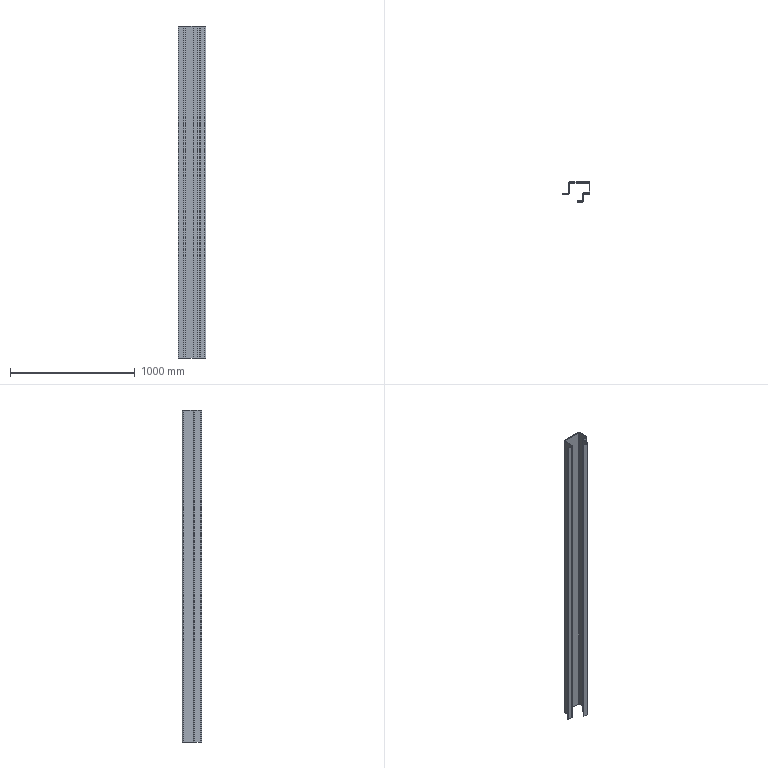Part | SolidWorks | features Extrusion 1 | 1 solid | 30 faces | box 224 x 158 x 2660 mm | volume 8679415 mm3 | plane 18 | cylinder 12 | commonest cylinder face diameters 12 x6 24 x6
STEP:
#1=CARTESIAN_POINT('',(-59.,158.,0.));
#2=VERTEX_POINT('',#1);
#3=CARTESIAN_POINT('',(-71.,146.,0.));
#4=VERTEX_POINT('',#3);
#5=CARTESIAN_POINT('',(-59.,146.,0.));
#6=DIRECTION('',(0.,0.,1.));
#7=DIRECTION('',(1.,0.,0.));
#8=AXIS2_PLACEMENT_3D('',#5,#6,#7);
#9=CIRCLE('',#8,12.);
#10=EDGE_CURVE('',#2,#4,#9,.T.);
#11=ORIENTED_EDGE('',*,*,#10,.T.);
#12=CARTESIAN_POINT('',(-71.,146.,2660.));
#13=VERTEX_POINT('',#12);
#14=CARTESIAN_POINT('',(-71.,146.,2660.));
#15=DIRECTION('',(0.,0.,-1.));
#16=VECTOR('',#15,1000.);
#17=LINE('',#14,#16);
#18=EDGE_CURVE('',#13,#4,#17,.T.);
#19=ORIENTED_EDGE('',*,*,#18,.F.);
#20=CARTESIAN_POINT('',(-59.,158.,2660.));
#21=VERTEX_POINT('',#20);
#22=CARTESIAN_POINT('',(-59.,146.,2660.));
#23=DIRECTION('',(0.,0.,1.));
#24=DIRECTION('',(1.,0.,0.));
#25=AXIS2_PLACEMENT_3D('',#22,#23,#24);
#26=CIRCLE('',#25,12.);
#27=EDGE_CURVE('',#21,#13,#26,.T.);
#28=ORIENTED_EDGE('',*,*,#27,.F.);
#29=CARTESIAN_POINT('',(-59.,158.,2660.));
#30=DIRECTION('',(0.,0.,-1.));
#31=VECTOR('',#30,1000.);
#32=LINE('',#29,#31);
#33=EDGE_CURVE('',#21,#2,#32,.T.);
#34=ORIENTED_EDGE('',*,*,#33,.T.);
#35=EDGE_LOOP('',(#11,#19,#28,#34));
#36=FACE_OUTER_BOUND('',#35,.T.);
#37=CARTESIAN_POINT('',(-59.,146.,2660.));
#38=DIRECTION('',(0.,0.,-1.));
#39=DIRECTION('',(-1.,0.,0.));
#40=AXIS2_PLACEMENT_3D('',#37,#38,#39);
#41=CYLINDRICAL_SURFACE('',#40,12.);
#42=ADVANCED_FACE('',(#36),#41,.T.);
#43=CARTESIAN_POINT('',(-71.,70.,0.));
#44=VERTEX_POINT('',#43);
#45=CARTESIAN_POINT('',(-71.,146.,0.));
#46=DIRECTION('',(0.,-1.,0.));
#47=VECTOR('',#46,1000.);
#48=LINE('',#45,#47);
#49=EDGE_CURVE('',#4,#44,#48,.T.);
#50=ORIENTED_EDGE('',*,*,#49,.T.);
#51=CARTESIAN_POINT('',(-71.,70.,2660.));
#52=VERTEX_POINT('',#51);
#53=CARTESIAN_POINT('',(-71.,70.,2660.));
#54=DIRECTION('',(0.,0.,-1.));
#55=VECTOR('',#54,1000.);
#56=LINE('',#53,#55);
#57=EDGE_CURVE('',#52,#44,#56,.T.);
#58=ORIENTED_EDGE('',*,*,#57,.F.);
#59=CARTESIAN_POINT('',(-71.,146.,2660.));
#60=DIRECTION('',(0.,-1.,0.));
#61=VECTOR('',#60,1000.);
#62=LINE('',#59,#61);
#63=EDGE_CURVE('',#13,#52,#62,.T.);
#64=ORIENTED_EDGE('',*,*,#63,.F.);
#65=ORIENTED_EDGE('',*,*,#18,.T.);
#66=EDGE_LOOP('',(#50,#58,#64,#65));
#67=FACE_OUTER_BOUND('',#66,.T.);
#68=CARTESIAN_POINT('',(-71.,146.,2660.));
#69=DIRECTION('',(1.,0.,0.));
#70=DIRECTION('',(0.,1.,0.));
#71=AXIS2_PLACEMENT_3D('',#68,#69,#70);
#72=PLANE('',#71);
#73=ADVANCED_FACE('',(#67),#72,.F.);
#74=CARTESIAN_POINT('',(-77.,64.,0.));
#75=VERTEX_POINT('',#74);
#76=CARTESIAN_POINT('',(-77.,70.,0.));
#77=DIRECTION('',(0.,0.,-1.));
#78=DIRECTION('',(1.,0.,0.));
#79=AXIS2_PLACEMENT_3D('',#76,#77,#78);
#80=CIRCLE('',#79,6.);
#81=EDGE_CURVE('',#44,#75,#80,.T.);
#82=ORIENTED_EDGE('',*,*,#81,.T.);
#83=CARTESIAN_POINT('',(-77.,64.,2660.));
#84=VERTEX_POINT('',#83);
#85=CARTESIAN_POINT('',(-77.,64.,2660.));
#86=DIRECTION('',(0.,0.,-1.));
#87=VECTOR('',#86,1000.);
#88=LINE('',#85,#87);
#89=EDGE_CURVE('',#84,#75,#88,.T.);
#90=ORIENTED_EDGE('',*,*,#89,.F.);
#91=CARTESIAN_POINT('',(-77.,70.,2660.));
#92=DIRECTION('',(0.,0.,-1.));
#93=DIRECTION('',(1.,0.,0.));
#94=AXIS2_PLACEMENT_3D('',#91,#92,#93);
#95=CIRCLE('',#94,6.);
#96=EDGE_CURVE('',#52,#84,#95,.T.);
#97=ORIENTED_EDGE('',*,*,#96,.F.);
#98=ORIENTED_EDGE('',*,*,#57,.T.);
#99=EDGE_LOOP('',(#82,#90,#97,#98));
#100=FACE_OUTER_BOUND('',#99,.T.);
#101=CARTESIAN_POINT('',(-77.,70.,2660.));
#102=DIRECTION('',(0.,0.,-1.));
#103=DIRECTION('',(-1.,0.,0.));
#104=AXIS2_PLACEMENT_3D('',#101,#102,#103);
#105=CYLINDRICAL_SURFACE('',#104,6.);
#106=ADVANCED_FACE('',(#100),#105,.F.);
#107=CARTESIAN_POINT('',(-121.,64.,0.));
#108=VERTEX_POINT('',#107);
#109=CARTESIAN_POINT('',(-77.,64.,0.));
#110=DIRECTION('',(-1.,0.,0.));
#111=VECTOR('',#110,1000.);
#112=LINE('',#109,#111);
#113=EDGE_CURVE('',#75,#108,#112,.T.);
#114=ORIENTED_EDGE('',*,*,#113,.T.);
#115=CARTESIAN_POINT('',(-121.,64.,2660.));
#116=VERTEX_POINT('',#115);
#117=CARTESIAN_POINT('',(-121.,64.,2660.));
#118=DIRECTION('',(0.,0.,-1.));
#119=VECTOR('',#118,1000.);
#120=LINE('',#117,#119);
#121=EDGE_CURVE('',#116,#108,#120,.T.);
#122=ORIENTED_EDGE('',*,*,#121,.F.);
#123=CARTESIAN_POINT('',(-77.,64.,2660.));
#124=DIRECTION('',(-1.,0.,0.));
#125=VECTOR('',#124,1000.);
#126=LINE('',#123,#125);
#127=EDGE_CURVE('',#84,#116,#126,.T.);
#128=ORIENTED_EDGE('',*,*,#127,.F.);
#129=ORIENTED_EDGE('',*,*,#89,.T.);
#130=EDGE_LOOP('',(#114,#122,#128,#129));
#131=FACE_OUTER_BOUND('',#130,.T.);
#132=CARTESIAN_POINT('',(-77.,64.,2660.));
#133=DIRECTION('',(0.,-1.,0.));
#134=DIRECTION('',(1.,0.,0.));
#135=AXIS2_PLACEMENT_3D('',#132,#133,#134);
#136=PLANE('',#135);
#137=ADVANCED_FACE('',(#131),#136,.F.);
#138=CARTESIAN_POINT('',(-121.,58.,0.));
#139=VERTEX_POINT('',#138);
#140=CARTESIAN_POINT('',(-121.,64.,0.));
#141=DIRECTION('',(0.,-1.,0.));
#142=VECTOR('',#141,1000.);
#143=LINE('',#140,#142);
#144=EDGE_CURVE('',#108,#139,#143,.T.);
#145=ORIENTED_EDGE('',*,*,#144,.T.);
#146=CARTESIAN_POINT('',(-121.,58.,2660.));
#147=VERTEX_POINT('',#146);
#148=CARTESIAN_POINT('',(-121.,58.,2660.));
#149=DIRECTION('',(0.,0.,-1.));
#150=VECTOR('',#149,1000.);
#151=LINE('',#148,#150);
#152=EDGE_CURVE('',#147,#139,#151,.T.);
#153=ORIENTED_EDGE('',*,*,#152,.F.);
#154=CARTESIAN_POINT('',(-121.,64.,2660.));
#155=DIRECTION('',(0.,-1.,0.));
#156=VECTOR('',#155,1000.);
#157=LINE('',#154,#156);
#158=EDGE_CURVE('',#116,#147,#157,.T.);
#159=ORIENTED_EDGE('',*,*,#158,.F.);
#160=ORIENTED_EDGE('',*,*,#121,.T.);
#161=EDGE_LOOP('',(#145,#153,#159,#160));
#162=FACE_OUTER_BOUND('',#161,.T.);
#163=CARTESIAN_POINT('',(-121.,64.,2660.));
#164=DIRECTION('',(1.,0.,0.));
#165=DIRECTION('',(0.,0.,-1.));
#166=AXIS2_PLACEMENT_3D('',#163,#164,#165);
#167=PLANE('',#166);
#168=ADVANCED_FACE('',(#162),#167,.F.);
#169=CARTESIAN_POINT('',(-77.,58.,0.));
#170=VERTEX_POINT('',#169);
#171=CARTESIAN_POINT('',(-121.,58.,0.));
#172=DIRECTION('',(1.,0.,0.));
#173=VECTOR('',#172,1000.);
#174=LINE('',#171,#173);
#175=EDGE_CURVE('',#139,#170,#174,.T.);
#176=ORIENTED_EDGE('',*,*,#175,.T.);
#177=CARTESIAN_POINT('',(-77.,58.,2660.));
#178=VERTEX_POINT('',#177);
#179=CARTESIAN_POINT('',(-77.,58.,2660.));
#180=DIRECTION('',(0.,0.,-1.));
#181=VECTOR('',#180,1000.);
#182=LINE('',#179,#181);
#183=EDGE_CURVE('',#178,#170,#182,.T.);
#184=ORIENTED_EDGE('',*,*,#183,.F.);
#185=CARTESIAN_POINT('',(-121.,58.,2660.));
#186=DIRECTION('',(1.,0.,0.));
#187=VECTOR('',#186,1000.);
#188=LINE('',#185,#187);
#189=EDGE_CURVE('',#147,#178,#188,.T.);
#190=ORIENTED_EDGE('',*,*,#189,.F.);
#191=ORIENTED_EDGE('',*,*,#152,.T.);
#192=EDGE_LOOP('',(#176,#184,#190,#191));
#193=FACE_OUTER_BOUND('',#192,.T.);
#194=CARTESIAN_POINT('',(-121.,58.,2660.));
#195=DIRECTION('',(0.,1.,0.));
#196=DIRECTION('',(0.,0.,1.));
#197=AXIS2_PLACEMENT_3D('',#194,#195,#196);
#198=PLANE('',#197);
#199=ADVANCED_FACE('',(#193),#198,.F.);
#200=CARTESIAN_POINT('',(-65.,70.,0.));
#201=VERTEX_POINT('',#200);
#202=CARTESIAN_POINT('',(-77.,70.,0.));
#203=DIRECTION('',(0.,0.,1.));
#204=DIRECTION('',(1.,0.,0.));
#205=AXIS2_PLACEMENT_3D('',#202,#203,#204);
#206=CIRCLE('',#205,12.);
#207=EDGE_CURVE('',#170,#201,#206,.T.);
#208=ORIENTED_EDGE('',*,*,#207,.T.);
#209=CARTESIAN_POINT('',(-65.,70.,2660.));
#210=VERTEX_POINT('',#209);
#211=CARTESIAN_POINT('',(-65.,70.,2660.));
#212=DIRECTION('',(0.,0.,-1.));
#213=VECTOR('',#212,1000.);
#214=LINE('',#211,#213);
#215=EDGE_CURVE('',#210,#201,#214,.T.);
#216=ORIENTED_EDGE('',*,*,#215,.F.);
#217=CARTESIAN_POINT('',(-77.,70.,2660.));
#218=DIRECTION('',(0.,0.,1.));
#219=DIRECTION('',(1.,0.,0.));
#220=AXIS2_PLACEMENT_3D('',#217,#218,#219);
#221=CIRCLE('',#220,12.);
#222=EDGE_CURVE('',#178,#210,#221,.T.);
#223=ORIENTED_EDGE('',*,*,#222,.F.);
#224=ORIENTED_EDGE('',*,*,#183,.T.);
#225=EDGE_LOOP('',(#208,#216,#223,#224));
#226=FACE_OUTER_BOUND('',#225,.T.);
#227=CARTESIAN_POINT('',(-77.,70.,2660.));
#228=DIRECTION('',(0.,0.,-1.));
#229=DIRECTION('',(-1.,0.,0.));
#230=AXIS2_PLACEMENT_3D('',#227,#228,#229);
#231=CYLINDRICAL_SURFACE('',#230,12.);
#232=ADVANCED_FACE('',(#226),#231,.T.);
#233=CARTESIAN_POINT('',(-65.,146.,0.));
#234=VERTEX_POINT('',#233);
#235=CARTESIAN_POINT('',(-65.,70.,0.));
#236=DIRECTION('',(0.,1.,0.));
#237=VECTOR('',#236,1000.);
#238=LINE('',#235,#237);
#239=EDGE_CURVE('',#201,#234,#238,.T.);
#240=ORIENTED_EDGE('',*,*,#239,.T.);
#241=CARTESIAN_POINT('',(-65.,146.,2660.));
#242=VERTEX_POINT('',#241);
#243=CARTESIAN_POINT('',(-65.,146.,2660.));
#244=DIRECTION('',(0.,0.,-1.));
#245=VECTOR('',#244,1000.);
#246=LINE('',#243,#245);
#247=EDGE_CURVE('',#242,#234,#246,.T.);
#248=ORIENTED_EDGE('',*,*,#247,.F.);
#249=CARTESIAN_POINT('',(-65.,70.,2660.));
#250=DIRECTION('',(0.,1.,0.));
#251=VECTOR('',#250,1000.);
#252=LINE('',#249,#251);
#253=EDGE_CURVE('',#210,#242,#252,.T.);
#254=ORIENTED_EDGE('',*,*,#253,.F.);
#255=ORIENTED_EDGE('',*,*,#215,.T.);
#256=EDGE_LOOP('',(#240,#248,#254,#255));
#257=FACE_OUTER_BOUND('',#256,.T.);
#258=CARTESIAN_POINT('',(-65.,70.,2660.));
#259=DIRECTION('',(-1.,0.,0.));
#260=DIRECTION('',(0.,0.,1.));
#261=AXIS2_PLACEMENT_3D('',#258,#259,#260);
#262=PLANE('',#261);
#263=ADVANCED_FACE('',(#257),#262,.F.);
#264=CARTESIAN_POINT('',(-59.,152.,0.));
#265=VERTEX_POINT('',#264);
#266=CARTESIAN_POINT('',(-59.,146.,0.));
#267=DIRECTION('',(0.,0.,-1.));
#268=DIRECTION('',(1.,0.,0.));
#269=AXIS2_PLACEMENT_3D('',#266,#267,#268);
#270=CIRCLE('',#269,6.);
#271=EDGE_CURVE('',#234,#265,#270,.T.);
#272=ORIENTED_EDGE('',*,*,#271,.T.);
#273=CARTESIAN_POINT('',(-59.,152.,2660.));
#274=VERTEX_POINT('',#273);
#275=CARTESIAN_POINT('',(-59.,152.,2660.));
#276=DIRECTION('',(0.,0.,-1.));
#277=VECTOR('',#276,1000.);
#278=LINE('',#275,#277);
#279=EDGE_CURVE('',#274,#265,#278,.T.);
#280=ORIENTED_EDGE('',*,*,#279,.F.);
#281=CARTESIAN_POINT('',(-59.,146.,2660.));
#282=DIRECTION('',(0.,0.,-1.));
#283=DIRECTION('',(1.,0.,0.));
#284=AXIS2_PLACEMENT_3D('',#281,#282,#283);
#285=CIRCLE('',#284,6.);
#286=EDGE_CURVE('',#242,#274,#285,.T.);
#287=ORIENTED_EDGE('',*,*,#286,.F.);
#288=ORIENTED_EDGE('',*,*,#247,.T.);
#289=EDGE_LOOP('',(#272,#280,#287,#288));
#290=FACE_OUTER_BOUND('',#289,.T.);
#291=CARTESIAN_POINT('',(-59.,146.,2660.));
#292=DIRECTION('',(0.,0.,-1.));
#293=DIRECTION('',(-1.,0.,0.));
#294=AXIS2_PLACEMENT_3D('',#291,#292,#293);
#295=CYLINDRICAL_SURFACE('',#294,6.);
#296=ADVANCED_FACE('',(#290),#295,.F.);
#297=CARTESIAN_POINT('',(91.,152.,0.));
#298=VERTEX_POINT('',#297);
#299=CARTESIAN_POINT('',(-59.,152.,0.));
#300=DIRECTION('',(1.,0.,0.));
#301=VECTOR('',#300,1000.);
#302=LINE('',#299,#301);
#303=EDGE_CURVE('',#265,#298,#302,.T.);
#304=ORIENTED_EDGE('',*,*,#303,.T.);
#305=CARTESIAN_POINT('',(91.,152.,2660.));
#306=VERTEX_POINT('',#305);
#307=CARTESIAN_POINT('',(91.,152.,2660.));
#308=DIRECTION('',(0.,0.,-1.));
#309=VECTOR('',#308,1000.);
#310=LINE('',#307,#309);
#311=EDGE_CURVE('',#306,#298,#310,.T.);
#312=ORIENTED_EDGE('',*,*,#311,.F.);
#313=CARTESIAN_POINT('',(-59.,152.,2660.));
#314=DIRECTION('',(1.,0.,0.));
#315=VECTOR('',#314,1000.);
#316=LINE('',#313,#315);
#317=EDGE_CURVE('',#274,#306,#316,.T.);
#318=ORIENTED_EDGE('',*,*,#317,.F.);
#319=ORIENTED_EDGE('',*,*,#279,.T.);
#320=EDGE_LOOP('',(#304,#312,#318,#319));
#321=FACE_OUTER_BOUND('',#320,.T.);
#322=CARTESIAN_POINT('',(-59.,152.,2660.));
#323=DIRECTION('',(0.,1.,0.));
#324=DIRECTION('',(0.,0.,1.));
#325=AXIS2_PLACEMENT_3D('',#322,#323,#324);
#326=PLANE('',#325);
#327=ADVANCED_FACE('',(#321),#326,.F.);
#328=CARTESIAN_POINT('',(97.,146.,0.));
#329=VERTEX_POINT('',#328);
#330=CARTESIAN_POINT('',(91.,146.,0.));
#331=DIRECTION('',(0.,0.,-1.));
#332=DIRECTION('',(1.,0.,0.));
#333=AXIS2_PLACEMENT_3D('',#330,#331,#332);
#334=CIRCLE('',#333,6.);
#335=EDGE_CURVE('',#298,#329,#334,.T.);
#336=ORIENTED_EDGE('',*,*,#335,.T.);
#337=CARTESIAN_POINT('',(97.,146.,2660.));
#338=VERTEX_POINT('',#337);
#339=CARTESIAN_POINT('',(97.,146.,2660.));
#340=DIRECTION('',(0.,0.,-1.));
#341=VECTOR('',#340,1000.);
#342=LINE('',#339,#341);
#343=EDGE_CURVE('',#338,#329,#342,.T.);
#344=ORIENTED_EDGE('',*,*,#343,.F.);
#345=CARTESIAN_POINT('',(91.,146.,2660.));
#346=DIRECTION('',(0.,0.,-1.));
#347=DIRECTION('',(1.,0.,0.));
#348=AXIS2_PLACEMENT_3D('',#345,#346,#347);
#349=CIRCLE('',#348,6.);
#350=EDGE_CURVE('',#306,#338,#349,.T.);
#351=ORIENTED_EDGE('',*,*,#350,.F.);
#352=ORIENTED_EDGE('',*,*,#311,.T.);
#353=EDGE_LOOP('',(#336,#344,#351,#352));
#354=FACE_OUTER_BOUND('',#353,.T.);
#355=CARTESIAN_POINT('',(91.,146.,2660.));
#356=DIRECTION('',(0.,0.,-1.));
#357=DIRECTION('',(-1.,0.,0.));
#358=AXIS2_PLACEMENT_3D('',#355,#356,#357);
#359=CYLINDRICAL_SURFACE('',#358,6.);
#360=ADVANCED_FACE('',(#354),#359,.F.);
#361=CARTESIAN_POINT('',(97.,76.,0.));
#362=VERTEX_POINT('',#361);
#363=CARTESIAN_POINT('',(97.,146.,0.));
#364=DIRECTION('',(0.,-1.,0.));
#365=VECTOR('',#364,1000.);
#366=LINE('',#363,#365);
#367=EDGE_CURVE('',#329,#362,#366,.T.);
#368=ORIENTED_EDGE('',*,*,#367,.T.);
#369=CARTESIAN_POINT('',(97.,76.,2660.));
#370=VERTEX_POINT('',#369);
#371=CARTESIAN_POINT('',(97.,76.,2660.));
#372=DIRECTION('',(0.,0.,-1.));
#373=VECTOR('',#372,1000.);
#374=LINE('',#371,#373);
#375=EDGE_CURVE('',#370,#362,#374,.T.);
#376=ORIENTED_EDGE('',*,*,#375,.F.);
#377=CARTESIAN_POINT('',(97.,146.,2660.));
#378=DIRECTION('',(0.,-1.,0.));
#379=VECTOR('',#378,1000.);
#380=LINE('',#377,#379);
#381=EDGE_CURVE('',#338,#370,#380,.T.);
#382=ORIENTED_EDGE('',*,*,#381,.F.);
#383=ORIENTED_EDGE('',*,*,#343,.T.);
#384=EDGE_LOOP('',(#368,#376,#382,#383));
#385=FACE_OUTER_BOUND('',#384,.T.);
#386=CARTESIAN_POINT('',(97.,146.,2660.));
#387=DIRECTION('',(1.,0.,0.));
#388=DIRECTION('',(0.,1.,0.));
#389=AXIS2_PLACEMENT_3D('',#386,#387,#388);
#390=PLANE('',#389);
#391=ADVANCED_FACE('',(#385),#390,.F.);
#392=CARTESIAN_POINT('',(91.,70.,0.));
#393=VERTEX_POINT('',#392);
#394=CARTESIAN_POINT('',(91.,76.,0.));
#395=DIRECTION('',(0.,0.,-1.));
#396=DIRECTION('',(1.,0.,0.));
#397=AXIS2_PLACEMENT_3D('',#394,#395,#396);
#398=CIRCLE('',#397,6.);
#399=EDGE_CURVE('',#362,#393,#398,.T.);
#400=ORIENTED_EDGE('',*,*,#399,.T.);
#401=CARTESIAN_POINT('',(91.,70.,2660.));
#402=VERTEX_POINT('',#401);
#403=CARTESIAN_POINT('',(91.,70.,2660.));
#404=DIRECTION('',(0.,0.,-1.));
#405=VECTOR('',#404,1000.);
#406=LINE('',#403,#405);
#407=EDGE_CURVE('',#402,#393,#406,.T.);
#408=ORIENTED_EDGE('',*,*,#407,.F.);
#409=CARTESIAN_POINT('',(91.,76.,2660.));
#410=DIRECTION('',(0.,0.,-1.));
#411=DIRECTION('',(1.,0.,0.));
#412=AXIS2_PLACEMENT_3D('',#409,#410,#411);
#413=CIRCLE('',#412,6.);
#414=EDGE_CURVE('',#370,#402,#413,.T.);
#415=ORIENTED_EDGE('',*,*,#414,.F.);
#416=ORIENTED_EDGE('',*,*,#375,.T.);
#417=EDGE_LOOP('',(#400,#408,#415,#416));
#418=FACE_OUTER_BOUND('',#417,.T.);
#419=CARTESIAN_POINT('',(91.,76.,2660.));
#420=DIRECTION('',(0.,0.,-1.));
#421=DIRECTION('',(-1.,0.,0.));
#422=AXIS2_PLACEMENT_3D('',#419,#420,#421);
#423=CYLINDRICAL_SURFACE('',#422,6.);
#424=ADVANCED_FACE('',(#418),#423,.F.);
#425=CARTESIAN_POINT('',(56.,70.,0.));
#426=VERTEX_POINT('',#425);
#427=CARTESIAN_POINT('',(91.,70.,0.));
#428=DIRECTION('',(-1.,0.,0.));
#429=VECTOR('',#428,1000.);
#430=LINE('',#427,#429);
#431=EDGE_CURVE('',#393,#426,#430,.T.);
#432=ORIENTED_EDGE('',*,*,#431,.T.);
#433=CARTESIAN_POINT('',(56.,70.,2660.));
#434=VERTEX_POINT('',#433);
#435=CARTESIAN_POINT('',(56.,70.,2660.));
#436=DIRECTION('',(0.,0.,-1.));
#437=VECTOR('',#436,1000.);
#438=LINE('',#435,#437);
#439=EDGE_CURVE('',#434,#426,#438,.T.);
#440=ORIENTED_EDGE('',*,*,#439,.F.);
#441=CARTESIAN_POINT('',(91.,70.,2660.));
#442=DIRECTION('',(-1.,0.,0.));
#443=VECTOR('',#442,1000.);
#444=LINE('',#441,#443);
#445=EDGE_CURVE('',#402,#434,#444,.T.);
#446=ORIENTED_EDGE('',*,*,#445,.F.);
#447=ORIENTED_EDGE('',*,*,#407,.T.);
#448=EDGE_LOOP('',(#432,#440,#446,#447));
#449=FACE_OUTER_BOUND('',#448,.T.);
#450=CARTESIAN_POINT('',(91.,70.,2660.));
#451=DIRECTION('',(0.,-1.,0.));
#452=DIRECTION('',(1.,0.,0.));
#453=AXIS2_PLACEMENT_3D('',#450,#451,#452);
#454=PLANE('',#453);
#455=ADVANCED_FACE('',(#449),#454,.F.);
#456=CARTESIAN_POINT('',(44.,58.,0.));
#457=VERTEX_POINT('',#456);
#458=CARTESIAN_POINT('',(56.,58.,0.));
#459=DIRECTION('',(0.,0.,1.));
#460=DIRECTION('',(1.,0.,0.));
#461=AXIS2_PLACEMENT_3D('',#458,#459,#460);
#462=CIRCLE('',#461,12.);
#463=EDGE_CURVE('',#426,#457,#462,.T.);
#464=ORIENTED_EDGE('',*,*,#463,.T.);
#465=CARTESIAN_POINT('',(44.,58.,2660.));
#466=VERTEX_POINT('',#465);
#467=CARTESIAN_POINT('',(44.,58.,2660.));
#468=DIRECTION('',(0.,0.,-1.));
#469=VECTOR('',#468,1000.);
#470=LINE('',#467,#469);
#471=EDGE_CURVE('',#466,#457,#470,.T.);
#472=ORIENTED_EDGE('',*,*,#471,.F.);
#473=CARTESIAN_POINT('',(56.,58.,2660.));
#474=DIRECTION('',(0.,0.,1.));
#475=DIRECTION('',(1.,0.,0.));
#476=AXIS2_PLACEMENT_3D('',#473,#474,#475);
#477=CIRCLE('',#476,12.);
#478=EDGE_CURVE('',#434,#466,#477,.T.);
#479=ORIENTED_EDGE('',*,*,#478,.F.);
#480=ORIENTED_EDGE('',*,*,#439,.T.);
#481=EDGE_LOOP('',(#464,#472,#479,#480));
#482=FACE_OUTER_BOUND('',#481,.T.);
#483=CARTESIAN_POINT('',(56.,58.,2660.));
#484=DIRECTION('',(0.,0.,-1.));
#485=DIRECTION('',(-1.,0.,0.));
#486=AXIS2_PLACEMENT_3D('',#483,#484,#485);
#487=CYLINDRICAL_SURFACE('',#486,12.);
#488=ADVANCED_FACE('',(#482),#487,.T.);
#489=CARTESIAN_POINT('',(44.,12.,0.));
#490=VERTEX_POINT('',#489);
#491=CARTESIAN_POINT('',(44.,58.,0.));
#492=DIRECTION('',(0.,-1.,0.));
#493=VECTOR('',#492,1000.);
#494=LINE('',#491,#493);
#495=EDGE_CURVE('',#457,#490,#494,.T.);
#496=ORIENTED_EDGE('',*,*,#495,.T.);
#497=CARTESIAN_POINT('',(44.,12.,2660.));
#498=VERTEX_POINT('',#497);
#499=CARTESIAN_POINT('',(44.,12.,2660.));
#500=DIRECTION('',(0.,0.,-1.));
#501=VECTOR('',#500,1000.);
#502=LINE('',#499,#501);
#503=EDGE_CURVE('',#498,#490,#502,.T.);
#504=ORIENTED_EDGE('',*,*,#503,.F.);
#505=CARTESIAN_POINT('',(44.,58.,2660.));
#506=DIRECTION('',(0.,-1.,0.));
#507=VECTOR('',#506,1000.);
#508=LINE('',#505,#507);
#509=EDGE_CURVE('',#466,#498,#508,.T.);
#510=ORIENTED_EDGE('',*,*,#509,.F.);
#511=ORIENTED_EDGE('',*,*,#471,.T.);
#512=EDGE_LOOP('',(#496,#504,#510,#511));
#513=FACE_OUTER_BOUND('',#512,.T.);
#514=CARTESIAN_POINT('',(44.,58.,2660.));
#515=DIRECTION('',(1.,0.,0.));
#516=DIRECTION('',(0.,1.,0.));
#517=AXIS2_PLACEMENT_3D('',#514,#515,#516);
#518=PLANE('',#517);
#519=ADVANCED_FACE('',(#513),#518,.F.);
#520=CARTESIAN_POINT('',(38.,6.,0.));
#521=VERTEX_POINT('',#520);
#522=CARTESIAN_POINT('',(38.,12.,0.));
#523=DIRECTION('',(0.,0.,-1.));
#524=DIRECTION('',(1.,0.,0.));
#525=AXIS2_PLACEMENT_3D('',#522,#523,#524);
#526=CIRCLE('',#525,6.);
#527=EDGE_CURVE('',#490,#521,#526,.T.);
#528=ORIENTED_EDGE('',*,*,#527,.T.);
#529=CARTESIAN_POINT('',(38.,6.,2660.));
#530=VERTEX_POINT('',#529);
#531=CARTESIAN_POINT('',(38.,6.,2660.));
#532=DIRECTION('',(0.,0.,-1.));
#533=VECTOR('',#532,1000.);
#534=LINE('',#531,#533);
#535=EDGE_CURVE('',#530,#521,#534,.T.);
#536=ORIENTED_EDGE('',*,*,#535,.F.);
#537=CARTESIAN_POINT('',(38.,12.,2660.));
#538=DIRECTION('',(0.,0.,-1.));
#539=DIRECTION('',(1.,0.,0.));
#540=AXIS2_PLACEMENT_3D('',#537,#538,#539);
#541=CIRCLE('',#540,6.);
#542=EDGE_CURVE('',#498,#530,#541,.T.);
#543=ORIENTED_EDGE('',*,*,#542,.F.);
#544=ORIENTED_EDGE('',*,*,#503,.T.);
#545=EDGE_LOOP('',(#528,#536,#543,#544));
#546=FACE_OUTER_BOUND('',#545,.T.);
#547=CARTESIAN_POINT('',(38.,12.,2660.));
#548=DIRECTION('',(0.,0.,-1.));
#549=DIRECTION('',(-1.,0.,0.));
#550=AXIS2_PLACEMENT_3D('',#547,#548,#549);
#551=CYLINDRICAL_SURFACE('',#550,6.);
#552=ADVANCED_FACE('',(#546),#551,.F.);
#553=CARTESIAN_POINT('',(0.,6.,0.));
#554=VERTEX_POINT('',#553);
#555=CARTESIAN_POINT('',(38.,6.,0.));
#556=DIRECTION('',(-1.,0.,0.));
#557=VECTOR('',#556,1000.);
#558=LINE('',#555,#557);
#559=EDGE_CURVE('',#521,#554,#558,.T.);
#560=ORIENTED_EDGE('',*,*,#559,.T.);
#561=CARTESIAN_POINT('',(0.,6.,2660.));
#562=VERTEX_POINT('',#561);
#563=CARTESIAN_POINT('',(0.,6.,2660.));
#564=DIRECTION('',(0.,0.,-1.));
#565=VECTOR('',#564,1000.);
#566=LINE('',#563,#565);
#567=EDGE_CURVE('',#562,#554,#566,.T.);
#568=ORIENTED_EDGE('',*,*,#567,.F.);
#569=CARTESIAN_POINT('',(38.,6.,2660.));
#570=DIRECTION('',(-1.,0.,0.));
#571=VECTOR('',#570,1000.);
#572=LINE('',#569,#571);
#573=EDGE_CURVE('',#530,#562,#572,.T.);
#574=ORIENTED_EDGE('',*,*,#573,.F.);
#575=ORIENTED_EDGE('',*,*,#535,.T.);
#576=EDGE_LOOP('',(#560,#568,#574,#575));
#577=FACE_OUTER_BOUND('',#576,.T.);
#578=CARTESIAN_POINT('',(38.,6.,2660.));
#579=DIRECTION('',(0.,-1.,0.));
#580=DIRECTION('',(1.,0.,0.));
#581=AXIS2_PLACEMENT_3D('',#578,#579,#580);
#582=PLANE('',#581);
#583=ADVANCED_FACE('',(#577),#582,.F.);
#584=CARTESIAN_POINT('',(0.,0.,0.));
#585=VERTEX_POINT('',#584);
#586=CARTESIAN_POINT('',(0.,6.,0.));
#587=DIRECTION('',(0.,-1.,0.));
#588=VECTOR('',#587,1000.);
#589=LINE('',#586,#588);
#590=EDGE_CURVE('',#554,#585,#589,.T.);
#591=ORIENTED_EDGE('',*,*,#590,.T.);
#592=CARTESIAN_POINT('',(0.,0.,2660.));
#593=VERTEX_POINT('',#592);
#594=CARTESIAN_POINT('',(0.,0.,2660.));
#595=DIRECTION('',(0.,0.,-1.));
#596=VECTOR('',#595,1000.);
#597=LINE('',#594,#596);
#598=EDGE_CURVE('',#593,#585,#597,.T.);
#599=ORIENTED_EDGE('',*,*,#598,.F.);
#600=CARTESIAN_POINT('',(0.,6.,2660.));
#601=DIRECTION('',(0.,-1.,0.));
#602=VECTOR('',#601,1000.);
#603=LINE('',#600,#602);
#604=EDGE_CURVE('',#562,#593,#603,.T.);
#605=ORIENTED_EDGE('',*,*,#604,.F.);
#606=ORIENTED_EDGE('',*,*,#567,.T.);
#607=EDGE_LOOP('',(#591,#599,#605,#606));
#608=FACE_OUTER_BOUND('',#607,.T.);
#609=CARTESIAN_POINT('',(0.,6.,2660.));
#610=DIRECTION('',(1.,0.,0.));
#611=DIRECTION('',(0.,0.,-1.));
#612=AXIS2_PLACEMENT_3D('',#609,#610,#611);
#613=PLANE('',#612);
#614=ADVANCED_FACE('',(#608),#613,.F.);
#615=CARTESIAN_POINT('',(38.,0.,0.));
#616=VERTEX_POINT('',#615);
#617=CARTESIAN_POINT('',(0.,0.,0.));
#618=DIRECTION('',(1.,0.,0.));
#619=VECTOR('',#618,1000.);
#620=LINE('',#617,#619);
#621=EDGE_CURVE('',#585,#616,#620,.T.);
#622=ORIENTED_EDGE('',*,*,#621,.T.);
#623=CARTESIAN_POINT('',(38.,0.,2660.));
#624=VERTEX_POINT('',#623);
#625=CARTESIAN_POINT('',(38.,0.,2660.));
#626=DIRECTION('',(0.,0.,-1.));
#627=VECTOR('',#626,1000.);
#628=LINE('',#625,#627);
#629=EDGE_CURVE('',#624,#616,#628,.T.);
#630=ORIENTED_EDGE('',*,*,#629,.F.);
#631=CARTESIAN_POINT('',(0.,0.,2660.));
#632=DIRECTION('',(1.,0.,0.));
#633=VECTOR('',#632,1000.);
#634=LINE('',#631,#633);
#635=EDGE_CURVE('',#593,#624,#634,.T.);
#636=ORIENTED_EDGE('',*,*,#635,.F.);
#637=ORIENTED_EDGE('',*,*,#598,.T.);
#638=EDGE_LOOP('',(#622,#630,#636,#637));
#639=FACE_OUTER_BOUND('',#638,.T.);
#640=CARTESIAN_POINT('',(0.,0.,2660.));
#641=DIRECTION('',(0.,1.,0.));
#642=DIRECTION('',(0.,0.,1.));
#643=AXIS2_PLACEMENT_3D('',#640,#641,#642);
#644=PLANE('',#643);
#645=ADVANCED_FACE('',(#639),#644,.F.);
#646=CARTESIAN_POINT('',(50.,12.,0.));
#647=VERTEX_POINT('',#646);
#648=CARTESIAN_POINT('',(38.,12.,0.));
#649=DIRECTION('',(0.,0.,1.));
#650=DIRECTION('',(1.,0.,0.));
#651=AXIS2_PLACEMENT_3D('',#648,#649,#650);
#652=CIRCLE('',#651,12.);
#653=EDGE_CURVE('',#616,#647,#652,.T.);
#654=ORIENTED_EDGE('',*,*,#653,.T.);
#655=CARTESIAN_POINT('',(50.,12.,2660.));
#656=VERTEX_POINT('',#655);
#657=CARTESIAN_POINT('',(50.,12.,2660.));
#658=DIRECTION('',(0.,0.,-1.));
#659=VECTOR('',#658,1000.);
#660=LINE('',#657,#659);
#661=EDGE_CURVE('',#656,#647,#660,.T.);
#662=ORIENTED_EDGE('',*,*,#661,.F.);
#663=CARTESIAN_POINT('',(38.,12.,2660.));
#664=DIRECTION('',(0.,0.,1.));
#665=DIRECTION('',(1.,0.,0.));
#666=AXIS2_PLACEMENT_3D('',#663,#664,#665);
#667=CIRCLE('',#666,12.);
#668=EDGE_CURVE('',#624,#656,#667,.T.);
#669=ORIENTED_EDGE('',*,*,#668,.F.);
#670=ORIENTED_EDGE('',*,*,#629,.T.);
#671=EDGE_LOOP('',(#654,#662,#669,#670));
#672=FACE_OUTER_BOUND('',#671,.T.);
#673=CARTESIAN_POINT('',(38.,12.,2660.));
#674=DIRECTION('',(0.,0.,-1.));
#675=DIRECTION('',(-1.,0.,0.));
#676=AXIS2_PLACEMENT_3D('',#673,#674,#675);
#677=CYLINDRICAL_SURFACE('',#676,12.);
#678=ADVANCED_FACE('',(#672),#677,.T.);
#679=CARTESIAN_POINT('',(50.,58.,0.));
#680=VERTEX_POINT('',#679);
#681=CARTESIAN_POINT('',(50.,12.,0.));
#682=DIRECTION('',(0.,1.,0.));
#683=VECTOR('',#682,1000.);
#684=LINE('',#681,#683);
#685=EDGE_CURVE('',#647,#680,#684,.T.);
#686=ORIENTED_EDGE('',*,*,#685,.T.);
#687=CARTESIAN_POINT('',(50.,58.,2660.));
#688=VERTEX_POINT('',#687);
#689=CARTESIAN_POINT('',(50.,58.,2660.));
#690=DIRECTION('',(0.,0.,-1.));
#691=VECTOR('',#690,1000.);
#692=LINE('',#689,#691);
#693=EDGE_CURVE('',#688,#680,#692,.T.);
#694=ORIENTED_EDGE('',*,*,#693,.F.);
#695=CARTESIAN_POINT('',(50.,12.,2660.));
#696=DIRECTION('',(0.,1.,0.));
#697=VECTOR('',#696,1000.);
#698=LINE('',#695,#697);
#699=EDGE_CURVE('',#656,#688,#698,.T.);
#700=ORIENTED_EDGE('',*,*,#699,.F.);
#701=ORIENTED_EDGE('',*,*,#661,.T.);
#702=EDGE_LOOP('',(#686,#694,#700,#701));
#703=FACE_OUTER_BOUND('',#702,.T.);
#704=CARTESIAN_POINT('',(50.,12.,2660.));
#705=DIRECTION('',(-1.,0.,0.));
#706=DIRECTION('',(0.,0.,1.));
#707=AXIS2_PLACEMENT_3D('',#704,#705,#706);
#708=PLANE('',#707);
#709=ADVANCED_FACE('',(#703),#708,.F.);
#710=CARTESIAN_POINT('',(56.,64.,0.));
#711=VERTEX_POINT('',#710);
#712=CARTESIAN_POINT('',(56.,58.,0.));
#713=DIRECTION('',(0.,0.,-1.));
#714=DIRECTION('',(1.,0.,0.));
#715=AXIS2_PLACEMENT_3D('',#712,#713,#714);
#716=CIRCLE('',#715,6.);
#717=EDGE_CURVE('',#680,#711,#716,.T.);
#718=ORIENTED_EDGE('',*,*,#717,.T.);
#719=CARTESIAN_POINT('',(56.,64.,2660.));
#720=VERTEX_POINT('',#719);
#721=CARTESIAN_POINT('',(56.,64.,2660.));
#722=DIRECTION('',(0.,0.,-1.));
#723=VECTOR('',#722,1000.);
#724=LINE('',#721,#723);
#725=EDGE_CURVE('',#720,#711,#724,.T.);
#726=ORIENTED_EDGE('',*,*,#725,.F.);
#727=CARTESIAN_POINT('',(56.,58.,2660.));
#728=DIRECTION('',(0.,0.,-1.));
#729=DIRECTION('',(1.,0.,0.));
#730=AXIS2_PLACEMENT_3D('',#727,#728,#729);
#731=CIRCLE('',#730,6.);
#732=EDGE_CURVE('',#688,#720,#731,.T.);
#733=ORIENTED_EDGE('',*,*,#732,.F.);
#734=ORIENTED_EDGE('',*,*,#693,.T.);
#735=EDGE_LOOP('',(#718,#726,#733,#734));
#736=FACE_OUTER_BOUND('',#735,.T.);
#737=CARTESIAN_POINT('',(56.,58.,2660.));
#738=DIRECTION('',(0.,0.,-1.));
#739=DIRECTION('',(-1.,0.,0.));
#740=AXIS2_PLACEMENT_3D('',#737,#738,#739);
#741=CYLINDRICAL_SURFACE('',#740,6.);
#742=ADVANCED_FACE('',(#736),#741,.F.);
#743=CARTESIAN_POINT('',(91.,64.,0.));
#744=VERTEX_POINT('',#743);
#745=CARTESIAN_POINT('',(56.,64.,0.));
#746=DIRECTION('',(1.,0.,0.));
#747=VECTOR('',#746,1000.);
#748=LINE('',#745,#747);
#749=EDGE_CURVE('',#711,#744,#748,.T.);
#750=ORIENTED_EDGE('',*,*,#749,.T.);
#751=CARTESIAN_POINT('',(91.,64.,2660.));
#752=VERTEX_POINT('',#751);
#753=CARTESIAN_POINT('',(91.,64.,2660.));
#754=DIRECTION('',(0.,0.,-1.));
#755=VECTOR('',#754,1000.);
#756=LINE('',#753,#755);
#757=EDGE_CURVE('',#752,#744,#756,.T.);
#758=ORIENTED_EDGE('',*,*,#757,.F.);
#759=CARTESIAN_POINT('',(56.,64.,2660.));
#760=DIRECTION('',(1.,0.,0.));
#761=VECTOR('',#760,1000.);
#762=LINE('',#759,#761);
#763=EDGE_CURVE('',#720,#752,#762,.T.);
#764=ORIENTED_EDGE('',*,*,#763,.F.);
#765=ORIENTED_EDGE('',*,*,#725,.T.);
#766=EDGE_LOOP('',(#750,#758,#764,#765));
#767=FACE_OUTER_BOUND('',#766,.T.);
#768=CARTESIAN_POINT('',(56.,64.,2660.));
#769=DIRECTION('',(0.,1.,0.));
#770=DIRECTION('',(-1.,0.,0.));
#771=AXIS2_PLACEMENT_3D('',#768,#769,#770);
#772=PLANE('',#771);
#773=ADVANCED_FACE('',(#767),#772,.F.);
#774=CARTESIAN_POINT('',(103.,76.,0.));
#775=VERTEX_POINT('',#774);
#776=CARTESIAN_POINT('',(91.,76.,0.));
#777=DIRECTION('',(0.,0.,1.));
#778=DIRECTION('',(1.,0.,0.));
#779=AXIS2_PLACEMENT_3D('',#776,#777,#778);
#780=CIRCLE('',#779,12.);
#781=EDGE_CURVE('',#744,#775,#780,.T.);
#782=ORIENTED_EDGE('',*,*,#781,.T.);
#783=CARTESIAN_POINT('',(103.,76.,2660.));
#784=VERTEX_POINT('',#783);
#785=CARTESIAN_POINT('',(103.,76.,2660.));
#786=DIRECTION('',(0.,0.,-1.));
#787=VECTOR('',#786,1000.);
#788=LINE('',#785,#787);
#789=EDGE_CURVE('',#784,#775,#788,.T.);
#790=ORIENTED_EDGE('',*,*,#789,.F.);
#791=CARTESIAN_POINT('',(91.,76.,2660.));
#792=DIRECTION('',(0.,0.,1.));
#793=DIRECTION('',(1.,0.,0.));
#794=AXIS2_PLACEMENT_3D('',#791,#792,#793);
#795=CIRCLE('',#794,12.);
#796=EDGE_CURVE('',#752,#784,#795,.T.);
#797=ORIENTED_EDGE('',*,*,#796,.F.);
#798=ORIENTED_EDGE('',*,*,#757,.T.);
#799=EDGE_LOOP('',(#782,#790,#797,#798));
#800=FACE_OUTER_BOUND('',#799,.T.);
#801=CARTESIAN_POINT('',(91.,76.,2660.));
#802=DIRECTION('',(0.,0.,-1.));
#803=DIRECTION('',(-1.,0.,0.));
#804=AXIS2_PLACEMENT_3D('',#801,#802,#803);
#805=CYLINDRICAL_SURFACE('',#804,12.);
#806=ADVANCED_FACE('',(#800),#805,.T.);
#807=CARTESIAN_POINT('',(103.,146.,0.));
#808=VERTEX_POINT('',#807);
#809=CARTESIAN_POINT('',(103.,76.,0.));
#810=DIRECTION('',(0.,1.,0.));
#811=VECTOR('',#810,1000.);
#812=LINE('',#809,#811);
#813=EDGE_CURVE('',#775,#808,#812,.T.);
#814=ORIENTED_EDGE('',*,*,#813,.T.);
#815=CARTESIAN_POINT('',(103.,146.,2660.));
#816=VERTEX_POINT('',#815);
#817=CARTESIAN_POINT('',(103.,146.,2660.));
#818=DIRECTION('',(0.,0.,-1.));
#819=VECTOR('',#818,1000.);
#820=LINE('',#817,#819);
#821=EDGE_CURVE('',#816,#808,#820,.T.);
#822=ORIENTED_EDGE('',*,*,#821,.F.);
#823=CARTESIAN_POINT('',(103.,76.,2660.));
#824=DIRECTION('',(0.,1.,0.));
#825=VECTOR('',#824,1000.);
#826=LINE('',#823,#825);
#827=EDGE_CURVE('',#784,#816,#826,.T.);
#828=ORIENTED_EDGE('',*,*,#827,.F.);
#829=ORIENTED_EDGE('',*,*,#789,.T.);
#830=EDGE_LOOP('',(#814,#822,#828,#829));
#831=FACE_OUTER_BOUND('',#830,.T.);
#832=CARTESIAN_POINT('',(103.,76.,2660.));
#833=DIRECTION('',(-1.,0.,0.));
#834=DIRECTION('',(0.,0.,1.));
#835=AXIS2_PLACEMENT_3D('',#832,#833,#834);
#836=PLANE('',#835);
#837=ADVANCED_FACE('',(#831),#836,.F.);
#838=CARTESIAN_POINT('',(91.,158.,0.));
#839=VERTEX_POINT('',#838);
#840=CARTESIAN_POINT('',(91.,146.,0.));
#841=DIRECTION('',(0.,0.,1.));
#842=DIRECTION('',(1.,0.,0.));
#843=AXIS2_PLACEMENT_3D('',#840,#841,#842);
#844=CIRCLE('',#843,12.);
#845=EDGE_CURVE('',#808,#839,#844,.T.);
#846=ORIENTED_EDGE('',*,*,#845,.T.);
#847=CARTESIAN_POINT('',(91.,158.,2660.));
#848=VERTEX_POINT('',#847);
#849=CARTESIAN_POINT('',(91.,158.,2660.));
#850=DIRECTION('',(0.,0.,-1.));
#851=VECTOR('',#850,1000.);
#852=LINE('',#849,#851);
#853=EDGE_CURVE('',#848,#839,#852,.T.);
#854=ORIENTED_EDGE('',*,*,#853,.F.);
#855=CARTESIAN_POINT('',(91.,146.,2660.));
#856=DIRECTION('',(0.,0.,1.));
#857=DIRECTION('',(1.,0.,0.));
#858=AXIS2_PLACEMENT_3D('',#855,#856,#857);
#859=CIRCLE('',#858,12.);
#860=EDGE_CURVE('',#816,#848,#859,.T.);
#861=ORIENTED_EDGE('',*,*,#860,.F.);
#862=ORIENTED_EDGE('',*,*,#821,.T.);
#863=EDGE_LOOP('',(#846,#854,#861,#862));
#864=FACE_OUTER_BOUND('',#863,.T.);
#865=CARTESIAN_POINT('',(91.,146.,2660.));
#866=DIRECTION('',(0.,0.,-1.));
#867=DIRECTION('',(-1.,0.,0.));
#868=AXIS2_PLACEMENT_3D('',#865,#866,#867);
#869=CYLINDRICAL_SURFACE('',#868,12.);
#870=ADVANCED_FACE('',(#864),#869,.T.);
#871=CARTESIAN_POINT('',(91.,158.,0.));
#872=DIRECTION('',(-1.,0.,0.));
#873=VECTOR('',#872,1000.);
#874=LINE('',#871,#873);
#875=EDGE_CURVE('',#839,#2,#874,.T.);
#876=ORIENTED_EDGE('',*,*,#875,.T.);
#877=ORIENTED_EDGE('',*,*,#33,.F.);
#878=CARTESIAN_POINT('',(91.,158.,2660.));
#879=DIRECTION('',(-1.,0.,0.));
#880=VECTOR('',#879,1000.);
#881=LINE('',#878,#880);
#882=EDGE_CURVE('',#848,#21,#881,.T.);
#883=ORIENTED_EDGE('',*,*,#882,.F.);
#884=ORIENTED_EDGE('',*,*,#853,.T.);
#885=EDGE_LOOP('',(#876,#877,#883,#884));
#886=FACE_OUTER_BOUND('',#885,.T.);
#887=CARTESIAN_POINT('',(91.,158.,2660.));
#888=DIRECTION('',(0.,-1.,0.));
#889=DIRECTION('',(1.,0.,0.));
#890=AXIS2_PLACEMENT_3D('',#887,#888,#889);
#891=PLANE('',#890);
#892=ADVANCED_FACE('',(#886),#891,.F.);
#893=ORIENTED_EDGE('',*,*,#27,.T.);
#894=ORIENTED_EDGE('',*,*,#63,.T.);
#895=ORIENTED_EDGE('',*,*,#96,.T.);
#896=ORIENTED_EDGE('',*,*,#127,.T.);
#897=ORIENTED_EDGE('',*,*,#158,.T.);
#898=ORIENTED_EDGE('',*,*,#189,.T.);
#899=ORIENTED_EDGE('',*,*,#222,.T.);
#900=ORIENTED_EDGE('',*,*,#253,.T.);
#901=ORIENTED_EDGE('',*,*,#286,.T.);
#902=ORIENTED_EDGE('',*,*,#317,.T.);
#903=ORIENTED_EDGE('',*,*,#350,.T.);
#904=ORIENTED_EDGE('',*,*,#381,.T.);
#905=ORIENTED_EDGE('',*,*,#414,.T.);
#906=ORIENTED_EDGE('',*,*,#445,.T.);
#907=ORIENTED_EDGE('',*,*,#478,.T.);
#908=ORIENTED_EDGE('',*,*,#509,.T.);
#909=ORIENTED_EDGE('',*,*,#542,.T.);
#910=ORIENTED_EDGE('',*,*,#573,.T.);
#911=ORIENTED_EDGE('',*,*,#604,.T.);
#912=ORIENTED_EDGE('',*,*,#635,.T.);
#913=ORIENTED_EDGE('',*,*,#668,.T.);
#914=ORIENTED_EDGE('',*,*,#699,.T.);
#915=ORIENTED_EDGE('',*,*,#732,.T.);
#916=ORIENTED_EDGE('',*,*,#763,.T.);
#917=ORIENTED_EDGE('',*,*,#796,.T.);
#918=ORIENTED_EDGE('',*,*,#827,.T.);
#919=ORIENTED_EDGE('',*,*,#860,.T.);
#920=ORIENTED_EDGE('',*,*,#882,.T.);
#921=EDGE_LOOP('',(#893,#894,#895,#896,#897,#898,#899,#900,#901,#902,#903,#904,#905,#906,#907,#908,#909,#910,#911,#912,#913,#914,#915,#916,#917,#918,#919,#920));
#922=FACE_OUTER_BOUND('',#921,.T.);
#923=CARTESIAN_POINT('',(-59.,146.,2660.));
#924=DIRECTION('',(0.,0.,1.));
#925=DIRECTION('',(1.,0.,0.));
#926=AXIS2_PLACEMENT_3D('',#923,#924,#925);
#927=PLANE('',#926);
#928=ADVANCED_FACE('',(#922),#927,.T.);
#929=ORIENTED_EDGE('',*,*,#10,.F.);
#930=ORIENTED_EDGE('',*,*,#875,.F.);
#931=ORIENTED_EDGE('',*,*,#845,.F.);
#932=ORIENTED_EDGE('',*,*,#813,.F.);
#933=ORIENTED_EDGE('',*,*,#781,.F.);
#934=ORIENTED_EDGE('',*,*,#749,.F.);
#935=ORIENTED_EDGE('',*,*,#717,.F.);
#936=ORIENTED_EDGE('',*,*,#685,.F.);
#937=ORIENTED_EDGE('',*,*,#653,.F.);
#938=ORIENTED_EDGE('',*,*,#621,.F.);
#939=ORIENTED_EDGE('',*,*,#590,.F.);
#940=ORIENTED_EDGE('',*,*,#559,.F.);
#941=ORIENTED_EDGE('',*,*,#527,.F.);
#942=ORIENTED_EDGE('',*,*,#495,.F.);
#943=ORIENTED_EDGE('',*,*,#463,.F.);
#944=ORIENTED_EDGE('',*,*,#431,.F.);
#945=ORIENTED_EDGE('',*,*,#399,.F.);
#946=ORIENTED_EDGE('',*,*,#367,.F.);
#947=ORIENTED_EDGE('',*,*,#335,.F.);
#948=ORIENTED_EDGE('',*,*,#303,.F.);
#949=ORIENTED_EDGE('',*,*,#271,.F.);
#950=ORIENTED_EDGE('',*,*,#239,.F.);
#951=ORIENTED_EDGE('',*,*,#207,.F.);
#952=ORIENTED_EDGE('',*,*,#175,.F.);
#953=ORIENTED_EDGE('',*,*,#144,.F.);
#954=ORIENTED_EDGE('',*,*,#113,.F.);
#955=ORIENTED_EDGE('',*,*,#81,.F.);
#956=ORIENTED_EDGE('',*,*,#49,.F.);
#957=EDGE_LOOP('',(#929,#930,#931,#932,#933,#934,#935,#936,#937,#938,#939,#940,#941,#942,#943,#944,#945,#946,#947,#948,#949,#950,#951,#952,#953,#954,#955,#956));
#958=FACE_OUTER_BOUND('',#957,.T.);
#959=CARTESIAN_POINT('',(-59.,146.,0.));
#960=DIRECTION('',(0.,0.,1.));
#961=DIRECTION('',(1.,0.,0.));
#962=AXIS2_PLACEMENT_3D('',#959,#960,#961);
#963=PLANE('',#962);
#964=ADVANCED_FACE('',(#958),#963,.F.);
#965=CLOSED_SHELL('',(#42,#73,#106,#137,#168,#199,#232,#263,#296,#327,#360,#391,#424,#455,#488,#519,#552,#583,#614,#645,#678,#709,#742,#773,#806,#837,#870,#892,#928,#964));
#966=MANIFOLD_SOLID_BREP('',#965);
#967=CARTESIAN_POINT('',(0.,0.,0.));
#968=DIRECTION('',(0.,0.,1.));
#969=DIRECTION('',(1.,0.,0.));
#970=AXIS2_PLACEMENT_3D('',#967,#968,#969);
#971=(LENGTH_UNIT()NAMED_UNIT(*)SI_UNIT(.MILLI.,.METRE.));
#972=UNCERTAINTY_MEASURE_WITH_UNIT(LENGTH_MEASURE(0.00001),#971,'','');
#973=(NAMED_UNIT(*)PLANE_ANGLE_UNIT()SI_UNIT($,.RADIAN.));
#974=(NAMED_UNIT(*)SI_UNIT($,.STERADIAN.)SOLID_ANGLE_UNIT());
#975=(GEOMETRIC_REPRESENTATION_CONTEXT(3)GLOBAL_UNCERTAINTY_ASSIGNED_CONTEXT((#972))GLOBAL_UNIT_ASSIGNED_CONTEXT((#971,#973,#974))REPRESENTATION_CONTEXT('',''));
#976=ADVANCED_BREP_SHAPE_REPRESENTATION('',(#966,#970),#975);